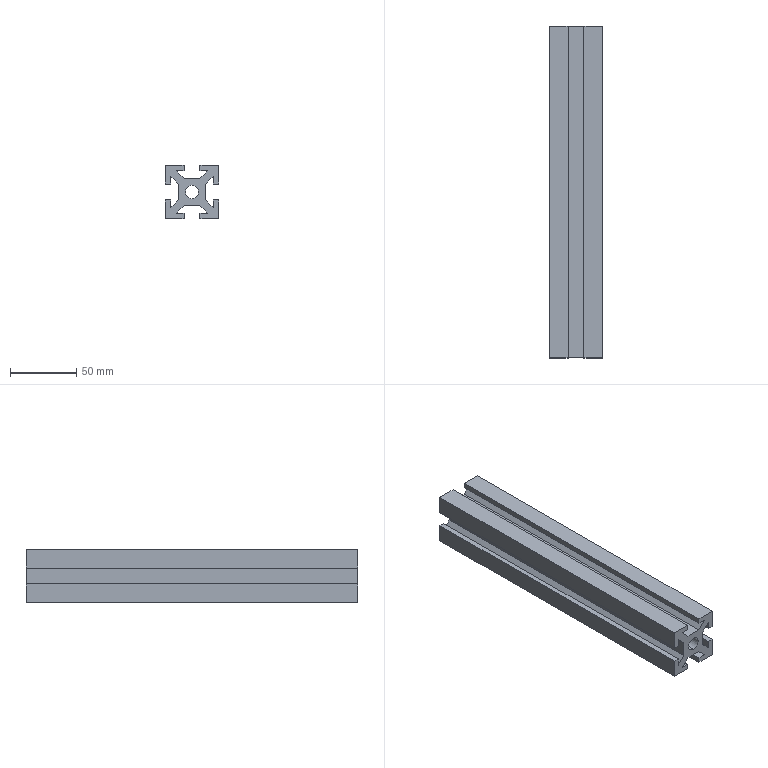Part | SolidWorks | features Extrusion 1 | 1 solid | 40 faces | box 40 x 250 x 40 mm | volume 227277 mm3 | plane 38 | cylinder 2 | commonest cylinder face diameters 10 x2
STEP:
#1=CARTESIAN_POINT('',(0.,250.,-5.));
#2=VERTEX_POINT('',#1);
#3=CARTESIAN_POINT('',(0.,250.,5.));
#4=VERTEX_POINT('',#3);
#5=CARTESIAN_POINT('',(0.,250.,0.));
#6=DIRECTION('',(0.,1.,0.));
#7=DIRECTION('',(0.,0.,1.));
#8=AXIS2_PLACEMENT_3D('',#5,#6,#7);
#9=CIRCLE('',#8,5.);
#10=EDGE_CURVE('',#2,#4,#9,.T.);
#11=ORIENTED_EDGE('',*,*,#10,.T.);
#12=CARTESIAN_POINT('',(0.,0.,5.));
#13=VERTEX_POINT('',#12);
#14=CARTESIAN_POINT('',(0.,250.,5.));
#15=DIRECTION('',(0.,-1.,0.));
#16=VECTOR('',#15,1000.);
#17=LINE('',#14,#16);
#18=EDGE_CURVE('',#4,#13,#17,.T.);
#19=ORIENTED_EDGE('',*,*,#18,.T.);
#20=CARTESIAN_POINT('',(0.,0.,-5.));
#21=VERTEX_POINT('',#20);
#22=CARTESIAN_POINT('',(0.,0.,0.));
#23=DIRECTION('',(0.,1.,0.));
#24=DIRECTION('',(0.,0.,1.));
#25=AXIS2_PLACEMENT_3D('',#22,#23,#24);
#26=CIRCLE('',#25,5.);
#27=EDGE_CURVE('',#21,#13,#26,.T.);
#28=ORIENTED_EDGE('',*,*,#27,.F.);
#29=CARTESIAN_POINT('',(0.,250.,-5.));
#30=DIRECTION('',(0.,-1.,0.));
#31=VECTOR('',#30,1000.);
#32=LINE('',#29,#31);
#33=EDGE_CURVE('',#2,#21,#32,.T.);
#34=ORIENTED_EDGE('',*,*,#33,.F.);
#35=EDGE_LOOP('',(#11,#19,#28,#34));
#36=FACE_OUTER_BOUND('',#35,.T.);
#37=CARTESIAN_POINT('',(0.,250.,0.));
#38=DIRECTION('',(0.,-1.,0.));
#39=DIRECTION('',(0.,0.,-1.));
#40=AXIS2_PLACEMENT_3D('',#37,#38,#39);
#41=CYLINDRICAL_SURFACE('',#40,5.);
#42=ADVANCED_FACE('',(#36),#41,.F.);
#43=CARTESIAN_POINT('',(6.,250.,20.));
#44=VERTEX_POINT('',#43);
#45=CARTESIAN_POINT('',(20.,250.,20.));
#46=VERTEX_POINT('',#45);
#47=CARTESIAN_POINT('',(6.,250.,20.));
#48=DIRECTION('',(1.,0.,0.));
#49=VECTOR('',#48,1000.);
#50=LINE('',#47,#49);
#51=EDGE_CURVE('',#44,#46,#50,.T.);
#52=ORIENTED_EDGE('',*,*,#51,.T.);
#53=CARTESIAN_POINT('',(20.,250.,6.));
#54=VERTEX_POINT('',#53);
#55=CARTESIAN_POINT('',(20.,250.,6.));
#56=DIRECTION('',(0.,0.,-1.));
#57=VECTOR('',#56,1000.);
#58=LINE('',#55,#57);
#59=EDGE_CURVE('',#46,#54,#58,.T.);
#60=ORIENTED_EDGE('',*,*,#59,.T.);
#61=CARTESIAN_POINT('',(16.,250.,6.));
#62=VERTEX_POINT('',#61);
#63=CARTESIAN_POINT('',(16.,250.,6.));
#64=DIRECTION('',(-1.,0.,0.));
#65=VECTOR('',#64,1000.);
#66=LINE('',#63,#65);
#67=EDGE_CURVE('',#54,#62,#66,.T.);
#68=ORIENTED_EDGE('',*,*,#67,.T.);
#69=CARTESIAN_POINT('',(16.,250.,11.757));
#70=VERTEX_POINT('',#69);
#71=CARTESIAN_POINT('',(16.,250.,11.757));
#72=DIRECTION('',(0.,0.,1.));
#73=VECTOR('',#72,1000.);
#74=LINE('',#71,#73);
#75=EDGE_CURVE('',#62,#70,#74,.T.);
#76=ORIENTED_EDGE('',*,*,#75,.T.);
#77=CARTESIAN_POINT('',(10.,250.,5.757));
#78=VERTEX_POINT('',#77);
#79=CARTESIAN_POINT('',(10.,250.,5.757));
#80=DIRECTION('',(-0.7071,0.,-0.7071));
#81=VECTOR('',#80,1000.);
#82=LINE('',#79,#81);
#83=EDGE_CURVE('',#70,#78,#82,.T.);
#84=ORIENTED_EDGE('',*,*,#83,.T.);
#85=CARTESIAN_POINT('',(10.,250.,-5.757));
#86=VERTEX_POINT('',#85);
#87=CARTESIAN_POINT('',(10.,250.,5.757));
#88=DIRECTION('',(0.,0.,-1.));
#89=VECTOR('',#88,1000.);
#90=LINE('',#87,#89);
#91=EDGE_CURVE('',#78,#86,#90,.T.);
#92=ORIENTED_EDGE('',*,*,#91,.T.);
#93=CARTESIAN_POINT('',(16.,250.,-11.757));
#94=VERTEX_POINT('',#93);
#95=CARTESIAN_POINT('',(16.,250.,-11.757));
#96=DIRECTION('',(0.7071,0.,-0.7071));
#97=VECTOR('',#96,1000.);
#98=LINE('',#95,#97);
#99=EDGE_CURVE('',#86,#94,#98,.T.);
#100=ORIENTED_EDGE('',*,*,#99,.T.);
#101=CARTESIAN_POINT('',(16.,250.,-6.));
#102=VERTEX_POINT('',#101);
#103=CARTESIAN_POINT('',(16.,250.,-6.));
#104=DIRECTION('',(0.,0.,1.));
#105=VECTOR('',#104,1000.);
#106=LINE('',#103,#105);
#107=EDGE_CURVE('',#94,#102,#106,.T.);
#108=ORIENTED_EDGE('',*,*,#107,.T.);
#109=CARTESIAN_POINT('',(20.,250.,-6.));
#110=VERTEX_POINT('',#109);
#111=CARTESIAN_POINT('',(20.,250.,-6.));
#112=DIRECTION('',(1.,0.,0.));
#113=VECTOR('',#112,1000.);
#114=LINE('',#111,#113);
#115=EDGE_CURVE('',#102,#110,#114,.T.);
#116=ORIENTED_EDGE('',*,*,#115,.T.);
#117=CARTESIAN_POINT('',(20.,250.,-20.));
#118=VERTEX_POINT('',#117);
#119=CARTESIAN_POINT('',(20.,250.,-20.));
#120=DIRECTION('',(0.,0.,-1.));
#121=VECTOR('',#120,1000.);
#122=LINE('',#119,#121);
#123=EDGE_CURVE('',#110,#118,#122,.T.);
#124=ORIENTED_EDGE('',*,*,#123,.T.);
#125=CARTESIAN_POINT('',(6.,250.,-20.));
#126=VERTEX_POINT('',#125);
#127=CARTESIAN_POINT('',(6.,250.,-20.));
#128=DIRECTION('',(-1.,0.,0.));
#129=VECTOR('',#128,1000.);
#130=LINE('',#127,#129);
#131=EDGE_CURVE('',#118,#126,#130,.T.);
#132=ORIENTED_EDGE('',*,*,#131,.T.);
#133=CARTESIAN_POINT('',(6.,250.,-16.));
#134=VERTEX_POINT('',#133);
#135=CARTESIAN_POINT('',(6.,250.,-16.));
#136=DIRECTION('',(0.,0.,1.));
#137=VECTOR('',#136,1000.);
#138=LINE('',#135,#137);
#139=EDGE_CURVE('',#126,#134,#138,.T.);
#140=ORIENTED_EDGE('',*,*,#139,.T.);
#141=CARTESIAN_POINT('',(11.757,250.,-16.));
#142=VERTEX_POINT('',#141);
#143=CARTESIAN_POINT('',(11.757,250.,-16.));
#144=DIRECTION('',(1.,0.,0.));
#145=VECTOR('',#144,1000.);
#146=LINE('',#143,#145);
#147=EDGE_CURVE('',#134,#142,#146,.T.);
#148=ORIENTED_EDGE('',*,*,#147,.T.);
#149=CARTESIAN_POINT('',(5.757,250.,-10.));
#150=VERTEX_POINT('',#149);
#151=CARTESIAN_POINT('',(5.757,250.,-10.));
#152=DIRECTION('',(-0.7071,0.,0.7071));
#153=VECTOR('',#152,1000.);
#154=LINE('',#151,#153);
#155=EDGE_CURVE('',#142,#150,#154,.T.);
#156=ORIENTED_EDGE('',*,*,#155,.T.);
#157=CARTESIAN_POINT('',(-5.757,250.,-10.));
#158=VERTEX_POINT('',#157);
#159=CARTESIAN_POINT('',(-5.757,250.,-10.));
#160=DIRECTION('',(-1.,0.,0.));
#161=VECTOR('',#160,1000.);
#162=LINE('',#159,#161);
#163=EDGE_CURVE('',#150,#158,#162,.T.);
#164=ORIENTED_EDGE('',*,*,#163,.T.);
#165=CARTESIAN_POINT('',(-11.757,250.,-16.));
#166=VERTEX_POINT('',#165);
#167=CARTESIAN_POINT('',(-11.757,250.,-16.));
#168=DIRECTION('',(-0.7071,0.,-0.7071));
#169=VECTOR('',#168,1000.);
#170=LINE('',#167,#169);
#171=EDGE_CURVE('',#158,#166,#170,.T.);
#172=ORIENTED_EDGE('',*,*,#171,.T.);
#173=CARTESIAN_POINT('',(-6.,250.,-16.));
#174=VERTEX_POINT('',#173);
#175=CARTESIAN_POINT('',(-6.,250.,-16.));
#176=DIRECTION('',(1.,0.,0.));
#177=VECTOR('',#176,1000.);
#178=LINE('',#175,#177);
#179=EDGE_CURVE('',#166,#174,#178,.T.);
#180=ORIENTED_EDGE('',*,*,#179,.T.);
#181=CARTESIAN_POINT('',(-6.,250.,-20.));
#182=VERTEX_POINT('',#181);
#183=CARTESIAN_POINT('',(-6.,250.,-20.));
#184=DIRECTION('',(0.,0.,-1.));
#185=VECTOR('',#184,1000.);
#186=LINE('',#183,#185);
#187=EDGE_CURVE('',#174,#182,#186,.T.);
#188=ORIENTED_EDGE('',*,*,#187,.T.);
#189=CARTESIAN_POINT('',(-20.,250.,-20.));
#190=VERTEX_POINT('',#189);
#191=CARTESIAN_POINT('',(-20.,250.,-20.));
#192=DIRECTION('',(-1.,0.,0.));
#193=VECTOR('',#192,1000.);
#194=LINE('',#191,#193);
#195=EDGE_CURVE('',#182,#190,#194,.T.);
#196=ORIENTED_EDGE('',*,*,#195,.T.);
#197=CARTESIAN_POINT('',(-20.,250.,-6.));
#198=VERTEX_POINT('',#197);
#199=CARTESIAN_POINT('',(-20.,250.,-20.));
#200=DIRECTION('',(0.,0.,1.));
#201=VECTOR('',#200,1000.);
#202=LINE('',#199,#201);
#203=EDGE_CURVE('',#190,#198,#202,.T.);
#204=ORIENTED_EDGE('',*,*,#203,.T.);
#205=CARTESIAN_POINT('',(-16.,250.,-6.));
#206=VERTEX_POINT('',#205);
#207=CARTESIAN_POINT('',(-16.,250.,-6.));
#208=DIRECTION('',(1.,0.,0.));
#209=VECTOR('',#208,1000.);
#210=LINE('',#207,#209);
#211=EDGE_CURVE('',#198,#206,#210,.T.);
#212=ORIENTED_EDGE('',*,*,#211,.T.);
#213=CARTESIAN_POINT('',(-16.,250.,-11.757));
#214=VERTEX_POINT('',#213);
#215=CARTESIAN_POINT('',(-16.,250.,-11.757));
#216=DIRECTION('',(0.,0.,-1.));
#217=VECTOR('',#216,1000.);
#218=LINE('',#215,#217);
#219=EDGE_CURVE('',#206,#214,#218,.T.);
#220=ORIENTED_EDGE('',*,*,#219,.T.);
#221=CARTESIAN_POINT('',(-10.,250.,-5.757));
#222=VERTEX_POINT('',#221);
#223=CARTESIAN_POINT('',(-10.,250.,-5.757));
#224=DIRECTION('',(0.7071,0.,0.7071));
#225=VECTOR('',#224,1000.);
#226=LINE('',#223,#225);
#227=EDGE_CURVE('',#214,#222,#226,.T.);
#228=ORIENTED_EDGE('',*,*,#227,.T.);
#229=CARTESIAN_POINT('',(-10.,250.,5.757));
#230=VERTEX_POINT('',#229);
#231=CARTESIAN_POINT('',(-10.,250.,5.757));
#232=DIRECTION('',(0.,0.,1.));
#233=VECTOR('',#232,1000.);
#234=LINE('',#231,#233);
#235=EDGE_CURVE('',#222,#230,#234,.T.);
#236=ORIENTED_EDGE('',*,*,#235,.T.);
#237=CARTESIAN_POINT('',(-16.,250.,11.757));
#238=VERTEX_POINT('',#237);
#239=CARTESIAN_POINT('',(-16.,250.,11.757));
#240=DIRECTION('',(-0.7071,0.,0.7071));
#241=VECTOR('',#240,1000.);
#242=LINE('',#239,#241);
#243=EDGE_CURVE('',#230,#238,#242,.T.);
#244=ORIENTED_EDGE('',*,*,#243,.T.);
#245=CARTESIAN_POINT('',(-16.,250.,6.));
#246=VERTEX_POINT('',#245);
#247=CARTESIAN_POINT('',(-16.,250.,6.));
#248=DIRECTION('',(0.,0.,-1.));
#249=VECTOR('',#248,1000.);
#250=LINE('',#247,#249);
#251=EDGE_CURVE('',#238,#246,#250,.T.);
#252=ORIENTED_EDGE('',*,*,#251,.T.);
#253=CARTESIAN_POINT('',(-20.,250.,6.));
#254=VERTEX_POINT('',#253);
#255=CARTESIAN_POINT('',(-20.,250.,6.));
#256=DIRECTION('',(-1.,0.,0.));
#257=VECTOR('',#256,1000.);
#258=LINE('',#255,#257);
#259=EDGE_CURVE('',#246,#254,#258,.T.);
#260=ORIENTED_EDGE('',*,*,#259,.T.);
#261=CARTESIAN_POINT('',(-20.,250.,20.));
#262=VERTEX_POINT('',#261);
#263=CARTESIAN_POINT('',(-20.,250.,6.));
#264=DIRECTION('',(0.,0.,1.));
#265=VECTOR('',#264,1000.);
#266=LINE('',#263,#265);
#267=EDGE_CURVE('',#254,#262,#266,.T.);
#268=ORIENTED_EDGE('',*,*,#267,.T.);
#269=CARTESIAN_POINT('',(-6.,250.,20.));
#270=VERTEX_POINT('',#269);
#271=CARTESIAN_POINT('',(-20.,250.,20.));
#272=DIRECTION('',(1.,0.,0.));
#273=VECTOR('',#272,1000.);
#274=LINE('',#271,#273);
#275=EDGE_CURVE('',#262,#270,#274,.T.);
#276=ORIENTED_EDGE('',*,*,#275,.T.);
#277=CARTESIAN_POINT('',(-6.,250.,16.));
#278=VERTEX_POINT('',#277);
#279=CARTESIAN_POINT('',(-6.,250.,16.));
#280=DIRECTION('',(0.,0.,-1.));
#281=VECTOR('',#280,1000.);
#282=LINE('',#279,#281);
#283=EDGE_CURVE('',#270,#278,#282,.T.);
#284=ORIENTED_EDGE('',*,*,#283,.T.);
#285=CARTESIAN_POINT('',(-11.757,250.,16.));
#286=VERTEX_POINT('',#285);
#287=CARTESIAN_POINT('',(-11.757,250.,16.));
#288=DIRECTION('',(-1.,0.,0.));
#289=VECTOR('',#288,1000.);
#290=LINE('',#287,#289);
#291=EDGE_CURVE('',#278,#286,#290,.T.);
#292=ORIENTED_EDGE('',*,*,#291,.T.);
#293=CARTESIAN_POINT('',(-5.757,250.,10.));
#294=VERTEX_POINT('',#293);
#295=CARTESIAN_POINT('',(-5.757,250.,10.));
#296=DIRECTION('',(0.7071,0.,-0.7071));
#297=VECTOR('',#296,1000.);
#298=LINE('',#295,#297);
#299=EDGE_CURVE('',#286,#294,#298,.T.);
#300=ORIENTED_EDGE('',*,*,#299,.T.);
#301=CARTESIAN_POINT('',(5.757,250.,10.));
#302=VERTEX_POINT('',#301);
#303=CARTESIAN_POINT('',(-5.757,250.,10.));
#304=DIRECTION('',(1.,0.,0.));
#305=VECTOR('',#304,1000.);
#306=LINE('',#303,#305);
#307=EDGE_CURVE('',#294,#302,#306,.T.);
#308=ORIENTED_EDGE('',*,*,#307,.T.);
#309=CARTESIAN_POINT('',(11.757,250.,16.));
#310=VERTEX_POINT('',#309);
#311=CARTESIAN_POINT('',(11.757,250.,16.));
#312=DIRECTION('',(0.7071,0.,0.7071));
#313=VECTOR('',#312,1000.);
#314=LINE('',#311,#313);
#315=EDGE_CURVE('',#302,#310,#314,.T.);
#316=ORIENTED_EDGE('',*,*,#315,.T.);
#317=CARTESIAN_POINT('',(6.,250.,16.));
#318=VERTEX_POINT('',#317);
#319=CARTESIAN_POINT('',(6.,250.,16.));
#320=DIRECTION('',(-1.,0.,0.));
#321=VECTOR('',#320,1000.);
#322=LINE('',#319,#321);
#323=EDGE_CURVE('',#310,#318,#322,.T.);
#324=ORIENTED_EDGE('',*,*,#323,.T.);
#325=CARTESIAN_POINT('',(6.,250.,20.));
#326=DIRECTION('',(0.,0.,1.));
#327=VECTOR('',#326,1000.);
#328=LINE('',#325,#327);
#329=EDGE_CURVE('',#318,#44,#328,.T.);
#330=ORIENTED_EDGE('',*,*,#329,.T.);
#331=EDGE_LOOP('',(#52,#60,#68,#76,#84,#92,#100,#108,#116,#124,#132,#140,#148,#156,#164,#172,#180,#188,#196,#204,#212,#220,#228,#236,#244,#252,#260,#268,#276,#284,#292,#300,#308,#316,#324,#330));
#332=FACE_OUTER_BOUND('',#331,.T.);
#333=ORIENTED_EDGE('',*,*,#10,.F.);
#334=CARTESIAN_POINT('',(0.,250.,0.));
#335=DIRECTION('',(0.,1.,0.));
#336=DIRECTION('',(0.,0.,1.));
#337=AXIS2_PLACEMENT_3D('',#334,#335,#336);
#338=CIRCLE('',#337,5.);
#339=EDGE_CURVE('',#4,#2,#338,.T.);
#340=ORIENTED_EDGE('',*,*,#339,.F.);
#341=EDGE_LOOP('',(#333,#340));
#342=FACE_BOUND('',#341,.T.);
#343=CARTESIAN_POINT('',(0.,250.,0.));
#344=DIRECTION('',(0.,-1.,0.));
#345=DIRECTION('',(0.,0.,-1.));
#346=AXIS2_PLACEMENT_3D('',#343,#344,#345);
#347=PLANE('',#346);
#348=ADVANCED_FACE('',(#332,#342),#347,.F.);
#349=CARTESIAN_POINT('',(6.,0.,20.));
#350=VERTEX_POINT('',#349);
#351=CARTESIAN_POINT('',(20.,0.,20.));
#352=VERTEX_POINT('',#351);
#353=CARTESIAN_POINT('',(6.,0.,20.));
#354=DIRECTION('',(1.,0.,0.));
#355=VECTOR('',#354,1000.);
#356=LINE('',#353,#355);
#357=EDGE_CURVE('',#350,#352,#356,.T.);
#358=ORIENTED_EDGE('',*,*,#357,.F.);
#359=CARTESIAN_POINT('',(6.,0.,16.));
#360=VERTEX_POINT('',#359);
#361=CARTESIAN_POINT('',(6.,0.,20.));
#362=DIRECTION('',(0.,0.,1.));
#363=VECTOR('',#362,1000.);
#364=LINE('',#361,#363);
#365=EDGE_CURVE('',#360,#350,#364,.T.);
#366=ORIENTED_EDGE('',*,*,#365,.F.);
#367=CARTESIAN_POINT('',(11.757,0.,16.));
#368=VERTEX_POINT('',#367);
#369=CARTESIAN_POINT('',(6.,0.,16.));
#370=DIRECTION('',(-1.,0.,0.));
#371=VECTOR('',#370,1000.);
#372=LINE('',#369,#371);
#373=EDGE_CURVE('',#368,#360,#372,.T.);
#374=ORIENTED_EDGE('',*,*,#373,.F.);
#375=CARTESIAN_POINT('',(5.757,0.,10.));
#376=VERTEX_POINT('',#375);
#377=CARTESIAN_POINT('',(11.757,0.,16.));
#378=DIRECTION('',(0.7071,0.,0.7071));
#379=VECTOR('',#378,1000.);
#380=LINE('',#377,#379);
#381=EDGE_CURVE('',#376,#368,#380,.T.);
#382=ORIENTED_EDGE('',*,*,#381,.F.);
#383=CARTESIAN_POINT('',(-5.757,0.,10.));
#384=VERTEX_POINT('',#383);
#385=CARTESIAN_POINT('',(-5.757,0.,10.));
#386=DIRECTION('',(1.,0.,0.));
#387=VECTOR('',#386,1000.);
#388=LINE('',#385,#387);
#389=EDGE_CURVE('',#384,#376,#388,.T.);
#390=ORIENTED_EDGE('',*,*,#389,.F.);
#391=CARTESIAN_POINT('',(-11.757,0.,16.));
#392=VERTEX_POINT('',#391);
#393=CARTESIAN_POINT('',(-5.757,0.,10.));
#394=DIRECTION('',(0.7071,0.,-0.7071));
#395=VECTOR('',#394,1000.);
#396=LINE('',#393,#395);
#397=EDGE_CURVE('',#392,#384,#396,.T.);
#398=ORIENTED_EDGE('',*,*,#397,.F.);
#399=CARTESIAN_POINT('',(-6.,0.,16.));
#400=VERTEX_POINT('',#399);
#401=CARTESIAN_POINT('',(-11.757,0.,16.));
#402=DIRECTION('',(-1.,0.,0.));
#403=VECTOR('',#402,1000.);
#404=LINE('',#401,#403);
#405=EDGE_CURVE('',#400,#392,#404,.T.);
#406=ORIENTED_EDGE('',*,*,#405,.F.);
#407=CARTESIAN_POINT('',(-6.,0.,20.));
#408=VERTEX_POINT('',#407);
#409=CARTESIAN_POINT('',(-6.,0.,16.));
#410=DIRECTION('',(0.,0.,-1.));
#411=VECTOR('',#410,1000.);
#412=LINE('',#409,#411);
#413=EDGE_CURVE('',#408,#400,#412,.T.);
#414=ORIENTED_EDGE('',*,*,#413,.F.);
#415=CARTESIAN_POINT('',(-20.,0.,20.));
#416=VERTEX_POINT('',#415);
#417=CARTESIAN_POINT('',(-20.,0.,20.));
#418=DIRECTION('',(1.,0.,0.));
#419=VECTOR('',#418,1000.);
#420=LINE('',#417,#419);
#421=EDGE_CURVE('',#416,#408,#420,.T.);
#422=ORIENTED_EDGE('',*,*,#421,.F.);
#423=CARTESIAN_POINT('',(-20.,0.,6.));
#424=VERTEX_POINT('',#423);
#425=CARTESIAN_POINT('',(-20.,0.,6.));
#426=DIRECTION('',(0.,0.,1.));
#427=VECTOR('',#426,1000.);
#428=LINE('',#425,#427);
#429=EDGE_CURVE('',#424,#416,#428,.T.);
#430=ORIENTED_EDGE('',*,*,#429,.F.);
#431=CARTESIAN_POINT('',(-16.,0.,6.));
#432=VERTEX_POINT('',#431);
#433=CARTESIAN_POINT('',(-20.,0.,6.));
#434=DIRECTION('',(-1.,0.,0.));
#435=VECTOR('',#434,1000.);
#436=LINE('',#433,#435);
#437=EDGE_CURVE('',#432,#424,#436,.T.);
#438=ORIENTED_EDGE('',*,*,#437,.F.);
#439=CARTESIAN_POINT('',(-16.,0.,11.757));
#440=VERTEX_POINT('',#439);
#441=CARTESIAN_POINT('',(-16.,0.,6.));
#442=DIRECTION('',(0.,0.,-1.));
#443=VECTOR('',#442,1000.);
#444=LINE('',#441,#443);
#445=EDGE_CURVE('',#440,#432,#444,.T.);
#446=ORIENTED_EDGE('',*,*,#445,.F.);
#447=CARTESIAN_POINT('',(-10.,0.,5.757));
#448=VERTEX_POINT('',#447);
#449=CARTESIAN_POINT('',(-16.,0.,11.757));
#450=DIRECTION('',(-0.7071,0.,0.7071));
#451=VECTOR('',#450,1000.);
#452=LINE('',#449,#451);
#453=EDGE_CURVE('',#448,#440,#452,.T.);
#454=ORIENTED_EDGE('',*,*,#453,.F.);
#455=CARTESIAN_POINT('',(-10.,0.,-5.757));
#456=VERTEX_POINT('',#455);
#457=CARTESIAN_POINT('',(-10.,0.,5.757));
#458=DIRECTION('',(0.,0.,1.));
#459=VECTOR('',#458,1000.);
#460=LINE('',#457,#459);
#461=EDGE_CURVE('',#456,#448,#460,.T.);
#462=ORIENTED_EDGE('',*,*,#461,.F.);
#463=CARTESIAN_POINT('',(-16.,0.,-11.757));
#464=VERTEX_POINT('',#463);
#465=CARTESIAN_POINT('',(-10.,0.,-5.757));
#466=DIRECTION('',(0.7071,0.,0.7071));
#467=VECTOR('',#466,1000.);
#468=LINE('',#465,#467);
#469=EDGE_CURVE('',#464,#456,#468,.T.);
#470=ORIENTED_EDGE('',*,*,#469,.F.);
#471=CARTESIAN_POINT('',(-16.,0.,-6.));
#472=VERTEX_POINT('',#471);
#473=CARTESIAN_POINT('',(-16.,0.,-11.757));
#474=DIRECTION('',(0.,0.,-1.));
#475=VECTOR('',#474,1000.);
#476=LINE('',#473,#475);
#477=EDGE_CURVE('',#472,#464,#476,.T.);
#478=ORIENTED_EDGE('',*,*,#477,.F.);
#479=CARTESIAN_POINT('',(-20.,0.,-6.));
#480=VERTEX_POINT('',#479);
#481=CARTESIAN_POINT('',(-16.,0.,-6.));
#482=DIRECTION('',(1.,0.,0.));
#483=VECTOR('',#482,1000.);
#484=LINE('',#481,#483);
#485=EDGE_CURVE('',#480,#472,#484,.T.);
#486=ORIENTED_EDGE('',*,*,#485,.F.);
#487=CARTESIAN_POINT('',(-20.,0.,-20.));
#488=VERTEX_POINT('',#487);
#489=CARTESIAN_POINT('',(-20.,0.,-20.));
#490=DIRECTION('',(0.,0.,1.));
#491=VECTOR('',#490,1000.);
#492=LINE('',#489,#491);
#493=EDGE_CURVE('',#488,#480,#492,.T.);
#494=ORIENTED_EDGE('',*,*,#493,.F.);
#495=CARTESIAN_POINT('',(-6.,0.,-20.));
#496=VERTEX_POINT('',#495);
#497=CARTESIAN_POINT('',(-20.,0.,-20.));
#498=DIRECTION('',(-1.,0.,0.));
#499=VECTOR('',#498,1000.);
#500=LINE('',#497,#499);
#501=EDGE_CURVE('',#496,#488,#500,.T.);
#502=ORIENTED_EDGE('',*,*,#501,.F.);
#503=CARTESIAN_POINT('',(-6.,0.,-16.));
#504=VERTEX_POINT('',#503);
#505=CARTESIAN_POINT('',(-6.,0.,-20.));
#506=DIRECTION('',(0.,0.,-1.));
#507=VECTOR('',#506,1000.);
#508=LINE('',#505,#507);
#509=EDGE_CURVE('',#504,#496,#508,.T.);
#510=ORIENTED_EDGE('',*,*,#509,.F.);
#511=CARTESIAN_POINT('',(-11.757,0.,-16.));
#512=VERTEX_POINT('',#511);
#513=CARTESIAN_POINT('',(-6.,0.,-16.));
#514=DIRECTION('',(1.,0.,0.));
#515=VECTOR('',#514,1000.);
#516=LINE('',#513,#515);
#517=EDGE_CURVE('',#512,#504,#516,.T.);
#518=ORIENTED_EDGE('',*,*,#517,.F.);
#519=CARTESIAN_POINT('',(-5.757,0.,-10.));
#520=VERTEX_POINT('',#519);
#521=CARTESIAN_POINT('',(-11.757,0.,-16.));
#522=DIRECTION('',(-0.7071,0.,-0.7071));
#523=VECTOR('',#522,1000.);
#524=LINE('',#521,#523);
#525=EDGE_CURVE('',#520,#512,#524,.T.);
#526=ORIENTED_EDGE('',*,*,#525,.F.);
#527=CARTESIAN_POINT('',(5.757,0.,-10.));
#528=VERTEX_POINT('',#527);
#529=CARTESIAN_POINT('',(-5.757,0.,-10.));
#530=DIRECTION('',(-1.,0.,0.));
#531=VECTOR('',#530,1000.);
#532=LINE('',#529,#531);
#533=EDGE_CURVE('',#528,#520,#532,.T.);
#534=ORIENTED_EDGE('',*,*,#533,.F.);
#535=CARTESIAN_POINT('',(11.757,0.,-16.));
#536=VERTEX_POINT('',#535);
#537=CARTESIAN_POINT('',(5.757,0.,-10.));
#538=DIRECTION('',(-0.7071,0.,0.7071));
#539=VECTOR('',#538,1000.);
#540=LINE('',#537,#539);
#541=EDGE_CURVE('',#536,#528,#540,.T.);
#542=ORIENTED_EDGE('',*,*,#541,.F.);
#543=CARTESIAN_POINT('',(6.,0.,-16.));
#544=VERTEX_POINT('',#543);
#545=CARTESIAN_POINT('',(11.757,0.,-16.));
#546=DIRECTION('',(1.,0.,0.));
#547=VECTOR('',#546,1000.);
#548=LINE('',#545,#547);
#549=EDGE_CURVE('',#544,#536,#548,.T.);
#550=ORIENTED_EDGE('',*,*,#549,.F.);
#551=CARTESIAN_POINT('',(6.,0.,-20.));
#552=VERTEX_POINT('',#551);
#553=CARTESIAN_POINT('',(6.,0.,-16.));
#554=DIRECTION('',(0.,0.,1.));
#555=VECTOR('',#554,1000.);
#556=LINE('',#553,#555);
#557=EDGE_CURVE('',#552,#544,#556,.T.);
#558=ORIENTED_EDGE('',*,*,#557,.F.);
#559=CARTESIAN_POINT('',(20.,0.,-20.));
#560=VERTEX_POINT('',#559);
#561=CARTESIAN_POINT('',(6.,0.,-20.));
#562=DIRECTION('',(-1.,0.,0.));
#563=VECTOR('',#562,1000.);
#564=LINE('',#561,#563);
#565=EDGE_CURVE('',#560,#552,#564,.T.);
#566=ORIENTED_EDGE('',*,*,#565,.F.);
#567=CARTESIAN_POINT('',(20.,0.,-6.));
#568=VERTEX_POINT('',#567);
#569=CARTESIAN_POINT('',(20.,0.,-20.));
#570=DIRECTION('',(0.,0.,-1.));
#571=VECTOR('',#570,1000.);
#572=LINE('',#569,#571);
#573=EDGE_CURVE('',#568,#560,#572,.T.);
#574=ORIENTED_EDGE('',*,*,#573,.F.);
#575=CARTESIAN_POINT('',(16.,0.,-6.));
#576=VERTEX_POINT('',#575);
#577=CARTESIAN_POINT('',(20.,0.,-6.));
#578=DIRECTION('',(1.,0.,0.));
#579=VECTOR('',#578,1000.);
#580=LINE('',#577,#579);
#581=EDGE_CURVE('',#576,#568,#580,.T.);
#582=ORIENTED_EDGE('',*,*,#581,.F.);
#583=CARTESIAN_POINT('',(16.,0.,-11.757));
#584=VERTEX_POINT('',#583);
#585=CARTESIAN_POINT('',(16.,0.,-6.));
#586=DIRECTION('',(0.,0.,1.));
#587=VECTOR('',#586,1000.);
#588=LINE('',#585,#587);
#589=EDGE_CURVE('',#584,#576,#588,.T.);
#590=ORIENTED_EDGE('',*,*,#589,.F.);
#591=CARTESIAN_POINT('',(10.,0.,-5.757));
#592=VERTEX_POINT('',#591);
#593=CARTESIAN_POINT('',(16.,0.,-11.757));
#594=DIRECTION('',(0.7071,0.,-0.7071));
#595=VECTOR('',#594,1000.);
#596=LINE('',#593,#595);
#597=EDGE_CURVE('',#592,#584,#596,.T.);
#598=ORIENTED_EDGE('',*,*,#597,.F.);
#599=CARTESIAN_POINT('',(10.,0.,5.757));
#600=VERTEX_POINT('',#599);
#601=CARTESIAN_POINT('',(10.,0.,5.757));
#602=DIRECTION('',(0.,0.,-1.));
#603=VECTOR('',#602,1000.);
#604=LINE('',#601,#603);
#605=EDGE_CURVE('',#600,#592,#604,.T.);
#606=ORIENTED_EDGE('',*,*,#605,.F.);
#607=CARTESIAN_POINT('',(16.,0.,11.757));
#608=VERTEX_POINT('',#607);
#609=CARTESIAN_POINT('',(10.,0.,5.757));
#610=DIRECTION('',(-0.7071,0.,-0.7071));
#611=VECTOR('',#610,1000.);
#612=LINE('',#609,#611);
#613=EDGE_CURVE('',#608,#600,#612,.T.);
#614=ORIENTED_EDGE('',*,*,#613,.F.);
#615=CARTESIAN_POINT('',(16.,0.,6.));
#616=VERTEX_POINT('',#615);
#617=CARTESIAN_POINT('',(16.,0.,11.757));
#618=DIRECTION('',(0.,0.,1.));
#619=VECTOR('',#618,1000.);
#620=LINE('',#617,#619);
#621=EDGE_CURVE('',#616,#608,#620,.T.);
#622=ORIENTED_EDGE('',*,*,#621,.F.);
#623=CARTESIAN_POINT('',(20.,0.,6.));
#624=VERTEX_POINT('',#623);
#625=CARTESIAN_POINT('',(16.,0.,6.));
#626=DIRECTION('',(-1.,0.,0.));
#627=VECTOR('',#626,1000.);
#628=LINE('',#625,#627);
#629=EDGE_CURVE('',#624,#616,#628,.T.);
#630=ORIENTED_EDGE('',*,*,#629,.F.);
#631=CARTESIAN_POINT('',(20.,0.,6.));
#632=DIRECTION('',(0.,0.,-1.));
#633=VECTOR('',#632,1000.);
#634=LINE('',#631,#633);
#635=EDGE_CURVE('',#352,#624,#634,.T.);
#636=ORIENTED_EDGE('',*,*,#635,.F.);
#637=EDGE_LOOP('',(#358,#366,#374,#382,#390,#398,#406,#414,#422,#430,#438,#446,#454,#462,#470,#478,#486,#494,#502,#510,#518,#526,#534,#542,#550,#558,#566,#574,#582,#590,#598,#606,#614,#622,#630,#636));
#638=FACE_OUTER_BOUND('',#637,.T.);
#639=ORIENTED_EDGE('',*,*,#27,.T.);
#640=CARTESIAN_POINT('',(0.,0.,0.));
#641=DIRECTION('',(0.,1.,0.));
#642=DIRECTION('',(0.,0.,1.));
#643=AXIS2_PLACEMENT_3D('',#640,#641,#642);
#644=CIRCLE('',#643,5.);
#645=EDGE_CURVE('',#13,#21,#644,.T.);
#646=ORIENTED_EDGE('',*,*,#645,.T.);
#647=EDGE_LOOP('',(#639,#646));
#648=FACE_BOUND('',#647,.T.);
#649=CARTESIAN_POINT('',(0.,0.,0.));
#650=DIRECTION('',(0.,-1.,0.));
#651=DIRECTION('',(0.,0.,-1.));
#652=AXIS2_PLACEMENT_3D('',#649,#650,#651);
#653=PLANE('',#652);
#654=ADVANCED_FACE('',(#638,#648),#653,.T.);
#655=ORIENTED_EDGE('',*,*,#357,.T.);
#656=CARTESIAN_POINT('',(20.,250.,20.));
#657=DIRECTION('',(0.,-1.,0.));
#658=VECTOR('',#657,1000.);
#659=LINE('',#656,#658);
#660=EDGE_CURVE('',#46,#352,#659,.T.);
#661=ORIENTED_EDGE('',*,*,#660,.F.);
#662=ORIENTED_EDGE('',*,*,#51,.F.);
#663=CARTESIAN_POINT('',(6.,250.,20.));
#664=DIRECTION('',(0.,-1.,0.));
#665=VECTOR('',#664,1000.);
#666=LINE('',#663,#665);
#667=EDGE_CURVE('',#44,#350,#666,.T.);
#668=ORIENTED_EDGE('',*,*,#667,.T.);
#669=EDGE_LOOP('',(#655,#661,#662,#668));
#670=FACE_OUTER_BOUND('',#669,.T.);
#671=CARTESIAN_POINT('',(6.,250.,20.));
#672=DIRECTION('',(0.,0.,-1.));
#673=DIRECTION('',(-1.,0.,0.));
#674=AXIS2_PLACEMENT_3D('',#671,#672,#673);
#675=PLANE('',#674);
#676=ADVANCED_FACE('',(#670),#675,.F.);
#677=ORIENTED_EDGE('',*,*,#635,.T.);
#678=CARTESIAN_POINT('',(20.,250.,6.));
#679=DIRECTION('',(0.,-1.,0.));
#680=VECTOR('',#679,1000.);
#681=LINE('',#678,#680);
#682=EDGE_CURVE('',#54,#624,#681,.T.);
#683=ORIENTED_EDGE('',*,*,#682,.F.);
#684=ORIENTED_EDGE('',*,*,#59,.F.);
#685=ORIENTED_EDGE('',*,*,#660,.T.);
#686=EDGE_LOOP('',(#677,#683,#684,#685));
#687=FACE_OUTER_BOUND('',#686,.T.);
#688=CARTESIAN_POINT('',(20.,250.,6.));
#689=DIRECTION('',(-1.,0.,0.));
#690=DIRECTION('',(0.,0.,1.));
#691=AXIS2_PLACEMENT_3D('',#688,#689,#690);
#692=PLANE('',#691);
#693=ADVANCED_FACE('',(#687),#692,.F.);
#694=ORIENTED_EDGE('',*,*,#629,.T.);
#695=CARTESIAN_POINT('',(16.,250.,6.));
#696=DIRECTION('',(0.,-1.,0.));
#697=VECTOR('',#696,1000.);
#698=LINE('',#695,#697);
#699=EDGE_CURVE('',#62,#616,#698,.T.);
#700=ORIENTED_EDGE('',*,*,#699,.F.);
#701=ORIENTED_EDGE('',*,*,#67,.F.);
#702=ORIENTED_EDGE('',*,*,#682,.T.);
#703=EDGE_LOOP('',(#694,#700,#701,#702));
#704=FACE_OUTER_BOUND('',#703,.T.);
#705=CARTESIAN_POINT('',(16.,250.,6.));
#706=DIRECTION('',(0.,0.,1.));
#707=DIRECTION('',(1.,0.,0.));
#708=AXIS2_PLACEMENT_3D('',#705,#706,#707);
#709=PLANE('',#708);
#710=ADVANCED_FACE('',(#704),#709,.F.);
#711=ORIENTED_EDGE('',*,*,#621,.T.);
#712=CARTESIAN_POINT('',(16.,250.,11.757));
#713=DIRECTION('',(0.,-1.,0.));
#714=VECTOR('',#713,1000.);
#715=LINE('',#712,#714);
#716=EDGE_CURVE('',#70,#608,#715,.T.);
#717=ORIENTED_EDGE('',*,*,#716,.F.);
#718=ORIENTED_EDGE('',*,*,#75,.F.);
#719=ORIENTED_EDGE('',*,*,#699,.T.);
#720=EDGE_LOOP('',(#711,#717,#718,#719));
#721=FACE_OUTER_BOUND('',#720,.T.);
#722=CARTESIAN_POINT('',(16.,250.,11.757));
#723=DIRECTION('',(1.,0.,0.));
#724=DIRECTION('',(0.,0.,-1.));
#725=AXIS2_PLACEMENT_3D('',#722,#723,#724);
#726=PLANE('',#725);
#727=ADVANCED_FACE('',(#721),#726,.F.);
#728=ORIENTED_EDGE('',*,*,#613,.T.);
#729=CARTESIAN_POINT('',(10.,250.,5.757));
#730=DIRECTION('',(0.,-1.,0.));
#731=VECTOR('',#730,1000.);
#732=LINE('',#729,#731);
#733=EDGE_CURVE('',#78,#600,#732,.T.);
#734=ORIENTED_EDGE('',*,*,#733,.F.);
#735=ORIENTED_EDGE('',*,*,#83,.F.);
#736=ORIENTED_EDGE('',*,*,#716,.T.);
#737=EDGE_LOOP('',(#728,#734,#735,#736));
#738=FACE_OUTER_BOUND('',#737,.T.);
#739=CARTESIAN_POINT('',(10.,250.,5.757));
#740=DIRECTION('',(-0.7071,0.,0.7071));
#741=DIRECTION('',(0.7071,0.,0.7071));
#742=AXIS2_PLACEMENT_3D('',#739,#740,#741);
#743=PLANE('',#742);
#744=ADVANCED_FACE('',(#738),#743,.F.);
#745=ORIENTED_EDGE('',*,*,#605,.T.);
#746=CARTESIAN_POINT('',(10.,250.,-5.757));
#747=DIRECTION('',(0.,-1.,0.));
#748=VECTOR('',#747,1000.);
#749=LINE('',#746,#748);
#750=EDGE_CURVE('',#86,#592,#749,.T.);
#751=ORIENTED_EDGE('',*,*,#750,.F.);
#752=ORIENTED_EDGE('',*,*,#91,.F.);
#753=ORIENTED_EDGE('',*,*,#733,.T.);
#754=EDGE_LOOP('',(#745,#751,#752,#753));
#755=FACE_OUTER_BOUND('',#754,.T.);
#756=CARTESIAN_POINT('',(10.,250.,5.757));
#757=DIRECTION('',(-1.,0.,0.));
#758=DIRECTION('',(0.,0.,1.));
#759=AXIS2_PLACEMENT_3D('',#756,#757,#758);
#760=PLANE('',#759);
#761=ADVANCED_FACE('',(#755),#760,.F.);
#762=ORIENTED_EDGE('',*,*,#597,.T.);
#763=CARTESIAN_POINT('',(16.,250.,-11.757));
#764=DIRECTION('',(0.,-1.,0.));
#765=VECTOR('',#764,1000.);
#766=LINE('',#763,#765);
#767=EDGE_CURVE('',#94,#584,#766,.T.);
#768=ORIENTED_EDGE('',*,*,#767,.F.);
#769=ORIENTED_EDGE('',*,*,#99,.F.);
#770=ORIENTED_EDGE('',*,*,#750,.T.);
#771=EDGE_LOOP('',(#762,#768,#769,#770));
#772=FACE_OUTER_BOUND('',#771,.T.);
#773=CARTESIAN_POINT('',(16.,250.,-11.757));
#774=DIRECTION('',(-0.7071,0.,-0.7071));
#775=DIRECTION('',(-0.7071,0.,0.7071));
#776=AXIS2_PLACEMENT_3D('',#773,#774,#775);
#777=PLANE('',#776);
#778=ADVANCED_FACE('',(#772),#777,.F.);
#779=ORIENTED_EDGE('',*,*,#589,.T.);
#780=CARTESIAN_POINT('',(16.,250.,-6.));
#781=DIRECTION('',(0.,-1.,0.));
#782=VECTOR('',#781,1000.);
#783=LINE('',#780,#782);
#784=EDGE_CURVE('',#102,#576,#783,.T.);
#785=ORIENTED_EDGE('',*,*,#784,.F.);
#786=ORIENTED_EDGE('',*,*,#107,.F.);
#787=ORIENTED_EDGE('',*,*,#767,.T.);
#788=EDGE_LOOP('',(#779,#785,#786,#787));
#789=FACE_OUTER_BOUND('',#788,.T.);
#790=CARTESIAN_POINT('',(16.,250.,-6.));
#791=DIRECTION('',(1.,0.,0.));
#792=DIRECTION('',(0.,0.,-1.));
#793=AXIS2_PLACEMENT_3D('',#790,#791,#792);
#794=PLANE('',#793);
#795=ADVANCED_FACE('',(#789),#794,.F.);
#796=ORIENTED_EDGE('',*,*,#581,.T.);
#797=CARTESIAN_POINT('',(20.,250.,-6.));
#798=DIRECTION('',(0.,-1.,0.));
#799=VECTOR('',#798,1000.);
#800=LINE('',#797,#799);
#801=EDGE_CURVE('',#110,#568,#800,.T.);
#802=ORIENTED_EDGE('',*,*,#801,.F.);
#803=ORIENTED_EDGE('',*,*,#115,.F.);
#804=ORIENTED_EDGE('',*,*,#784,.T.);
#805=EDGE_LOOP('',(#796,#802,#803,#804));
#806=FACE_OUTER_BOUND('',#805,.T.);
#807=CARTESIAN_POINT('',(20.,250.,-6.));
#808=DIRECTION('',(0.,0.,-1.));
#809=DIRECTION('',(-1.,0.,0.));
#810=AXIS2_PLACEMENT_3D('',#807,#808,#809);
#811=PLANE('',#810);
#812=ADVANCED_FACE('',(#806),#811,.F.);
#813=ORIENTED_EDGE('',*,*,#573,.T.);
#814=CARTESIAN_POINT('',(20.,250.,-20.));
#815=DIRECTION('',(0.,-1.,0.));
#816=VECTOR('',#815,1000.);
#817=LINE('',#814,#816);
#818=EDGE_CURVE('',#118,#560,#817,.T.);
#819=ORIENTED_EDGE('',*,*,#818,.F.);
#820=ORIENTED_EDGE('',*,*,#123,.F.);
#821=ORIENTED_EDGE('',*,*,#801,.T.);
#822=EDGE_LOOP('',(#813,#819,#820,#821));
#823=FACE_OUTER_BOUND('',#822,.T.);
#824=CARTESIAN_POINT('',(20.,250.,-20.));
#825=DIRECTION('',(-1.,0.,0.));
#826=DIRECTION('',(0.,0.,1.));
#827=AXIS2_PLACEMENT_3D('',#824,#825,#826);
#828=PLANE('',#827);
#829=ADVANCED_FACE('',(#823),#828,.F.);
#830=ORIENTED_EDGE('',*,*,#565,.T.);
#831=CARTESIAN_POINT('',(6.,250.,-20.));
#832=DIRECTION('',(0.,-1.,0.));
#833=VECTOR('',#832,1000.);
#834=LINE('',#831,#833);
#835=EDGE_CURVE('',#126,#552,#834,.T.);
#836=ORIENTED_EDGE('',*,*,#835,.F.);
#837=ORIENTED_EDGE('',*,*,#131,.F.);
#838=ORIENTED_EDGE('',*,*,#818,.T.);
#839=EDGE_LOOP('',(#830,#836,#837,#838));
#840=FACE_OUTER_BOUND('',#839,.T.);
#841=CARTESIAN_POINT('',(6.,250.,-20.));
#842=DIRECTION('',(0.,0.,1.));
#843=DIRECTION('',(1.,0.,0.));
#844=AXIS2_PLACEMENT_3D('',#841,#842,#843);
#845=PLANE('',#844);
#846=ADVANCED_FACE('',(#840),#845,.F.);
#847=ORIENTED_EDGE('',*,*,#557,.T.);
#848=CARTESIAN_POINT('',(6.,250.,-16.));
#849=DIRECTION('',(0.,-1.,0.));
#850=VECTOR('',#849,1000.);
#851=LINE('',#848,#850);
#852=EDGE_CURVE('',#134,#544,#851,.T.);
#853=ORIENTED_EDGE('',*,*,#852,.F.);
#854=ORIENTED_EDGE('',*,*,#139,.F.);
#855=ORIENTED_EDGE('',*,*,#835,.T.);
#856=EDGE_LOOP('',(#847,#853,#854,#855));
#857=FACE_OUTER_BOUND('',#856,.T.);
#858=CARTESIAN_POINT('',(6.,250.,-16.));
#859=DIRECTION('',(1.,0.,0.));
#860=DIRECTION('',(0.,0.,-1.));
#861=AXIS2_PLACEMENT_3D('',#858,#859,#860);
#862=PLANE('',#861);
#863=ADVANCED_FACE('',(#857),#862,.F.);
#864=ORIENTED_EDGE('',*,*,#549,.T.);
#865=CARTESIAN_POINT('',(11.757,250.,-16.));
#866=DIRECTION('',(0.,-1.,0.));
#867=VECTOR('',#866,1000.);
#868=LINE('',#865,#867);
#869=EDGE_CURVE('',#142,#536,#868,.T.);
#870=ORIENTED_EDGE('',*,*,#869,.F.);
#871=ORIENTED_EDGE('',*,*,#147,.F.);
#872=ORIENTED_EDGE('',*,*,#852,.T.);
#873=EDGE_LOOP('',(#864,#870,#871,#872));
#874=FACE_OUTER_BOUND('',#873,.T.);
#875=CARTESIAN_POINT('',(11.757,250.,-16.));
#876=DIRECTION('',(0.,0.,-1.));
#877=DIRECTION('',(-1.,0.,0.));
#878=AXIS2_PLACEMENT_3D('',#875,#876,#877);
#879=PLANE('',#878);
#880=ADVANCED_FACE('',(#874),#879,.F.);
#881=ORIENTED_EDGE('',*,*,#541,.T.);
#882=CARTESIAN_POINT('',(5.757,250.,-10.));
#883=DIRECTION('',(0.,-1.,0.));
#884=VECTOR('',#883,1000.);
#885=LINE('',#882,#884);
#886=EDGE_CURVE('',#150,#528,#885,.T.);
#887=ORIENTED_EDGE('',*,*,#886,.F.);
#888=ORIENTED_EDGE('',*,*,#155,.F.);
#889=ORIENTED_EDGE('',*,*,#869,.T.);
#890=EDGE_LOOP('',(#881,#887,#888,#889));
#891=FACE_OUTER_BOUND('',#890,.T.);
#892=CARTESIAN_POINT('',(5.757,250.,-10.));
#893=DIRECTION('',(0.7071,0.,0.7071));
#894=DIRECTION('',(0.7071,0.,-0.7071));
#895=AXIS2_PLACEMENT_3D('',#892,#893,#894);
#896=PLANE('',#895);
#897=ADVANCED_FACE('',(#891),#896,.F.);
#898=ORIENTED_EDGE('',*,*,#533,.T.);
#899=CARTESIAN_POINT('',(-5.757,250.,-10.));
#900=DIRECTION('',(0.,-1.,0.));
#901=VECTOR('',#900,1000.);
#902=LINE('',#899,#901);
#903=EDGE_CURVE('',#158,#520,#902,.T.);
#904=ORIENTED_EDGE('',*,*,#903,.F.);
#905=ORIENTED_EDGE('',*,*,#163,.F.);
#906=ORIENTED_EDGE('',*,*,#886,.T.);
#907=EDGE_LOOP('',(#898,#904,#905,#906));
#908=FACE_OUTER_BOUND('',#907,.T.);
#909=CARTESIAN_POINT('',(-5.757,250.,-10.));
#910=DIRECTION('',(0.,0.,1.));
#911=DIRECTION('',(1.,0.,0.));
#912=AXIS2_PLACEMENT_3D('',#909,#910,#911);
#913=PLANE('',#912);
#914=ADVANCED_FACE('',(#908),#913,.F.);
#915=ORIENTED_EDGE('',*,*,#525,.T.);
#916=CARTESIAN_POINT('',(-11.757,250.,-16.));
#917=DIRECTION('',(0.,-1.,0.));
#918=VECTOR('',#917,1000.);
#919=LINE('',#916,#918);
#920=EDGE_CURVE('',#166,#512,#919,.T.);
#921=ORIENTED_EDGE('',*,*,#920,.F.);
#922=ORIENTED_EDGE('',*,*,#171,.F.);
#923=ORIENTED_EDGE('',*,*,#903,.T.);
#924=EDGE_LOOP('',(#915,#921,#922,#923));
#925=FACE_OUTER_BOUND('',#924,.T.);
#926=CARTESIAN_POINT('',(-11.757,250.,-16.));
#927=DIRECTION('',(-0.7071,0.,0.7071));
#928=DIRECTION('',(0.7071,0.,0.7071));
#929=AXIS2_PLACEMENT_3D('',#926,#927,#928);
#930=PLANE('',#929);
#931=ADVANCED_FACE('',(#925),#930,.F.);
#932=ORIENTED_EDGE('',*,*,#517,.T.);
#933=CARTESIAN_POINT('',(-6.,250.,-16.));
#934=DIRECTION('',(0.,-1.,0.));
#935=VECTOR('',#934,1000.);
#936=LINE('',#933,#935);
#937=EDGE_CURVE('',#174,#504,#936,.T.);
#938=ORIENTED_EDGE('',*,*,#937,.F.);
#939=ORIENTED_EDGE('',*,*,#179,.F.);
#940=ORIENTED_EDGE('',*,*,#920,.T.);
#941=EDGE_LOOP('',(#932,#938,#939,#940));
#942=FACE_OUTER_BOUND('',#941,.T.);
#943=CARTESIAN_POINT('',(-6.,250.,-16.));
#944=DIRECTION('',(0.,0.,-1.));
#945=DIRECTION('',(-1.,0.,0.));
#946=AXIS2_PLACEMENT_3D('',#943,#944,#945);
#947=PLANE('',#946);
#948=ADVANCED_FACE('',(#942),#947,.F.);
#949=ORIENTED_EDGE('',*,*,#509,.T.);
#950=CARTESIAN_POINT('',(-6.,250.,-20.));
#951=DIRECTION('',(0.,-1.,0.));
#952=VECTOR('',#951,1000.);
#953=LINE('',#950,#952);
#954=EDGE_CURVE('',#182,#496,#953,.T.);
#955=ORIENTED_EDGE('',*,*,#954,.F.);
#956=ORIENTED_EDGE('',*,*,#187,.F.);
#957=ORIENTED_EDGE('',*,*,#937,.T.);
#958=EDGE_LOOP('',(#949,#955,#956,#957));
#959=FACE_OUTER_BOUND('',#958,.T.);
#960=CARTESIAN_POINT('',(-6.,250.,-20.));
#961=DIRECTION('',(-1.,0.,0.));
#962=DIRECTION('',(0.,0.,1.));
#963=AXIS2_PLACEMENT_3D('',#960,#961,#962);
#964=PLANE('',#963);
#965=ADVANCED_FACE('',(#959),#964,.F.);
#966=ORIENTED_EDGE('',*,*,#501,.T.);
#967=CARTESIAN_POINT('',(-20.,250.,-20.));
#968=DIRECTION('',(0.,-1.,0.));
#969=VECTOR('',#968,1000.);
#970=LINE('',#967,#969);
#971=EDGE_CURVE('',#190,#488,#970,.T.);
#972=ORIENTED_EDGE('',*,*,#971,.F.);
#973=ORIENTED_EDGE('',*,*,#195,.F.);
#974=ORIENTED_EDGE('',*,*,#954,.T.);
#975=EDGE_LOOP('',(#966,#972,#973,#974));
#976=FACE_OUTER_BOUND('',#975,.T.);
#977=CARTESIAN_POINT('',(-20.,250.,-20.));
#978=DIRECTION('',(0.,0.,1.));
#979=DIRECTION('',(1.,0.,0.));
#980=AXIS2_PLACEMENT_3D('',#977,#978,#979);
#981=PLANE('',#980);
#982=ADVANCED_FACE('',(#976),#981,.F.);
#983=ORIENTED_EDGE('',*,*,#493,.T.);
#984=CARTESIAN_POINT('',(-20.,250.,-6.));
#985=DIRECTION('',(0.,-1.,0.));
#986=VECTOR('',#985,1000.);
#987=LINE('',#984,#986);
#988=EDGE_CURVE('',#198,#480,#987,.T.);
#989=ORIENTED_EDGE('',*,*,#988,.F.);
#990=ORIENTED_EDGE('',*,*,#203,.F.);
#991=ORIENTED_EDGE('',*,*,#971,.T.);
#992=EDGE_LOOP('',(#983,#989,#990,#991));
#993=FACE_OUTER_BOUND('',#992,.T.);
#994=CARTESIAN_POINT('',(-20.,250.,-20.));
#995=DIRECTION('',(1.,0.,0.));
#996=DIRECTION('',(0.,0.,-1.));
#997=AXIS2_PLACEMENT_3D('',#994,#995,#996);
#998=PLANE('',#997);
#999=ADVANCED_FACE('',(#993),#998,.F.);
#1000=ORIENTED_EDGE('',*,*,#485,.T.);
#1001=CARTESIAN_POINT('',(-16.,250.,-6.));
#1002=DIRECTION('',(0.,-1.,0.));
#1003=VECTOR('',#1002,1000.);
#1004=LINE('',#1001,#1003);
#1005=EDGE_CURVE('',#206,#472,#1004,.T.);
#1006=ORIENTED_EDGE('',*,*,#1005,.F.);
#1007=ORIENTED_EDGE('',*,*,#211,.F.);
#1008=ORIENTED_EDGE('',*,*,#988,.T.);
#1009=EDGE_LOOP('',(#1000,#1006,#1007,#1008));
#1010=FACE_OUTER_BOUND('',#1009,.T.);
#1011=CARTESIAN_POINT('',(-16.,250.,-6.));
#1012=DIRECTION('',(0.,0.,-1.));
#1013=DIRECTION('',(-1.,0.,0.));
#1014=AXIS2_PLACEMENT_3D('',#1011,#1012,#1013);
#1015=PLANE('',#1014);
#1016=ADVANCED_FACE('',(#1010),#1015,.F.);
#1017=ORIENTED_EDGE('',*,*,#477,.T.);
#1018=CARTESIAN_POINT('',(-16.,250.,-11.757));
#1019=DIRECTION('',(0.,-1.,0.));
#1020=VECTOR('',#1019,1000.);
#1021=LINE('',#1018,#1020);
#1022=EDGE_CURVE('',#214,#464,#1021,.T.);
#1023=ORIENTED_EDGE('',*,*,#1022,.F.);
#1024=ORIENTED_EDGE('',*,*,#219,.F.);
#1025=ORIENTED_EDGE('',*,*,#1005,.T.);
#1026=EDGE_LOOP('',(#1017,#1023,#1024,#1025));
#1027=FACE_OUTER_BOUND('',#1026,.T.);
#1028=CARTESIAN_POINT('',(-16.,250.,-11.757));
#1029=DIRECTION('',(-1.,0.,0.));
#1030=DIRECTION('',(0.,0.,1.));
#1031=AXIS2_PLACEMENT_3D('',#1028,#1029,#1030);
#1032=PLANE('',#1031);
#1033=ADVANCED_FACE('',(#1027),#1032,.F.);
#1034=ORIENTED_EDGE('',*,*,#469,.T.);
#1035=CARTESIAN_POINT('',(-10.,250.,-5.757));
#1036=DIRECTION('',(0.,-1.,0.));
#1037=VECTOR('',#1036,1000.);
#1038=LINE('',#1035,#1037);
#1039=EDGE_CURVE('',#222,#456,#1038,.T.);
#1040=ORIENTED_EDGE('',*,*,#1039,.F.);
#1041=ORIENTED_EDGE('',*,*,#227,.F.);
#1042=ORIENTED_EDGE('',*,*,#1022,.T.);
#1043=EDGE_LOOP('',(#1034,#1040,#1041,#1042));
#1044=FACE_OUTER_BOUND('',#1043,.T.);
#1045=CARTESIAN_POINT('',(-10.,250.,-5.757));
#1046=DIRECTION('',(0.7071,0.,-0.7071));
#1047=DIRECTION('',(-0.7071,0.,-0.7071));
#1048=AXIS2_PLACEMENT_3D('',#1045,#1046,#1047);
#1049=PLANE('',#1048);
#1050=ADVANCED_FACE('',(#1044),#1049,.F.);
#1051=ORIENTED_EDGE('',*,*,#461,.T.);
#1052=CARTESIAN_POINT('',(-10.,250.,5.757));
#1053=DIRECTION('',(0.,-1.,0.));
#1054=VECTOR('',#1053,1000.);
#1055=LINE('',#1052,#1054);
#1056=EDGE_CURVE('',#230,#448,#1055,.T.);
#1057=ORIENTED_EDGE('',*,*,#1056,.F.);
#1058=ORIENTED_EDGE('',*,*,#235,.F.);
#1059=ORIENTED_EDGE('',*,*,#1039,.T.);
#1060=EDGE_LOOP('',(#1051,#1057,#1058,#1059));
#1061=FACE_OUTER_BOUND('',#1060,.T.);
#1062=CARTESIAN_POINT('',(-10.,250.,5.757));
#1063=DIRECTION('',(1.,0.,0.));
#1064=DIRECTION('',(0.,0.,-1.));
#1065=AXIS2_PLACEMENT_3D('',#1062,#1063,#1064);
#1066=PLANE('',#1065);
#1067=ADVANCED_FACE('',(#1061),#1066,.F.);
#1068=ORIENTED_EDGE('',*,*,#453,.T.);
#1069=CARTESIAN_POINT('',(-16.,250.,11.757));
#1070=DIRECTION('',(0.,-1.,0.));
#1071=VECTOR('',#1070,1000.);
#1072=LINE('',#1069,#1071);
#1073=EDGE_CURVE('',#238,#440,#1072,.T.);
#1074=ORIENTED_EDGE('',*,*,#1073,.F.);
#1075=ORIENTED_EDGE('',*,*,#243,.F.);
#1076=ORIENTED_EDGE('',*,*,#1056,.T.);
#1077=EDGE_LOOP('',(#1068,#1074,#1075,#1076));
#1078=FACE_OUTER_BOUND('',#1077,.T.);
#1079=CARTESIAN_POINT('',(-16.,250.,11.757));
#1080=DIRECTION('',(0.7071,0.,0.7071));
#1081=DIRECTION('',(0.7071,0.,-0.7071));
#1082=AXIS2_PLACEMENT_3D('',#1079,#1080,#1081);
#1083=PLANE('',#1082);
#1084=ADVANCED_FACE('',(#1078),#1083,.F.);
#1085=ORIENTED_EDGE('',*,*,#445,.T.);
#1086=CARTESIAN_POINT('',(-16.,250.,6.));
#1087=DIRECTION('',(0.,-1.,0.));
#1088=VECTOR('',#1087,1000.);
#1089=LINE('',#1086,#1088);
#1090=EDGE_CURVE('',#246,#432,#1089,.T.);
#1091=ORIENTED_EDGE('',*,*,#1090,.F.);
#1092=ORIENTED_EDGE('',*,*,#251,.F.);
#1093=ORIENTED_EDGE('',*,*,#1073,.T.);
#1094=EDGE_LOOP('',(#1085,#1091,#1092,#1093));
#1095=FACE_OUTER_BOUND('',#1094,.T.);
#1096=CARTESIAN_POINT('',(-16.,250.,6.));
#1097=DIRECTION('',(-1.,0.,0.));
#1098=DIRECTION('',(0.,0.,1.));
#1099=AXIS2_PLACEMENT_3D('',#1096,#1097,#1098);
#1100=PLANE('',#1099);
#1101=ADVANCED_FACE('',(#1095),#1100,.F.);
#1102=ORIENTED_EDGE('',*,*,#437,.T.);
#1103=CARTESIAN_POINT('',(-20.,250.,6.));
#1104=DIRECTION('',(0.,-1.,0.));
#1105=VECTOR('',#1104,1000.);
#1106=LINE('',#1103,#1105);
#1107=EDGE_CURVE('',#254,#424,#1106,.T.);
#1108=ORIENTED_EDGE('',*,*,#1107,.F.);
#1109=ORIENTED_EDGE('',*,*,#259,.F.);
#1110=ORIENTED_EDGE('',*,*,#1090,.T.);
#1111=EDGE_LOOP('',(#1102,#1108,#1109,#1110));
#1112=FACE_OUTER_BOUND('',#1111,.T.);
#1113=CARTESIAN_POINT('',(-20.,250.,6.));
#1114=DIRECTION('',(0.,0.,1.));
#1115=DIRECTION('',(1.,0.,0.));
#1116=AXIS2_PLACEMENT_3D('',#1113,#1114,#1115);
#1117=PLANE('',#1116);
#1118=ADVANCED_FACE('',(#1112),#1117,.F.);
#1119=ORIENTED_EDGE('',*,*,#429,.T.);
#1120=CARTESIAN_POINT('',(-20.,250.,20.));
#1121=DIRECTION('',(0.,-1.,0.));
#1122=VECTOR('',#1121,1000.);
#1123=LINE('',#1120,#1122);
#1124=EDGE_CURVE('',#262,#416,#1123,.T.);
#1125=ORIENTED_EDGE('',*,*,#1124,.F.);
#1126=ORIENTED_EDGE('',*,*,#267,.F.);
#1127=ORIENTED_EDGE('',*,*,#1107,.T.);
#1128=EDGE_LOOP('',(#1119,#1125,#1126,#1127));
#1129=FACE_OUTER_BOUND('',#1128,.T.);
#1130=CARTESIAN_POINT('',(-20.,250.,6.));
#1131=DIRECTION('',(1.,0.,0.));
#1132=DIRECTION('',(0.,0.,-1.));
#1133=AXIS2_PLACEMENT_3D('',#1130,#1131,#1132);
#1134=PLANE('',#1133);
#1135=ADVANCED_FACE('',(#1129),#1134,.F.);
#1136=ORIENTED_EDGE('',*,*,#421,.T.);
#1137=CARTESIAN_POINT('',(-6.,250.,20.));
#1138=DIRECTION('',(0.,-1.,0.));
#1139=VECTOR('',#1138,1000.);
#1140=LINE('',#1137,#1139);
#1141=EDGE_CURVE('',#270,#408,#1140,.T.);
#1142=ORIENTED_EDGE('',*,*,#1141,.F.);
#1143=ORIENTED_EDGE('',*,*,#275,.F.);
#1144=ORIENTED_EDGE('',*,*,#1124,.T.);
#1145=EDGE_LOOP('',(#1136,#1142,#1143,#1144));
#1146=FACE_OUTER_BOUND('',#1145,.T.);
#1147=CARTESIAN_POINT('',(-20.,250.,20.));
#1148=DIRECTION('',(0.,0.,-1.));
#1149=DIRECTION('',(-1.,0.,0.));
#1150=AXIS2_PLACEMENT_3D('',#1147,#1148,#1149);
#1151=PLANE('',#1150);
#1152=ADVANCED_FACE('',(#1146),#1151,.F.);
#1153=ORIENTED_EDGE('',*,*,#413,.T.);
#1154=CARTESIAN_POINT('',(-6.,250.,16.));
#1155=DIRECTION('',(0.,-1.,0.));
#1156=VECTOR('',#1155,1000.);
#1157=LINE('',#1154,#1156);
#1158=EDGE_CURVE('',#278,#400,#1157,.T.);
#1159=ORIENTED_EDGE('',*,*,#1158,.F.);
#1160=ORIENTED_EDGE('',*,*,#283,.F.);
#1161=ORIENTED_EDGE('',*,*,#1141,.T.);
#1162=EDGE_LOOP('',(#1153,#1159,#1160,#1161));
#1163=FACE_OUTER_BOUND('',#1162,.T.);
#1164=CARTESIAN_POINT('',(-6.,250.,16.));
#1165=DIRECTION('',(-1.,0.,0.));
#1166=DIRECTION('',(0.,0.,1.));
#1167=AXIS2_PLACEMENT_3D('',#1164,#1165,#1166);
#1168=PLANE('',#1167);
#1169=ADVANCED_FACE('',(#1163),#1168,.F.);
#1170=ORIENTED_EDGE('',*,*,#405,.T.);
#1171=CARTESIAN_POINT('',(-11.757,250.,16.));
#1172=DIRECTION('',(0.,-1.,0.));
#1173=VECTOR('',#1172,1000.);
#1174=LINE('',#1171,#1173);
#1175=EDGE_CURVE('',#286,#392,#1174,.T.);
#1176=ORIENTED_EDGE('',*,*,#1175,.F.);
#1177=ORIENTED_EDGE('',*,*,#291,.F.);
#1178=ORIENTED_EDGE('',*,*,#1158,.T.);
#1179=EDGE_LOOP('',(#1170,#1176,#1177,#1178));
#1180=FACE_OUTER_BOUND('',#1179,.T.);
#1181=CARTESIAN_POINT('',(-11.757,250.,16.));
#1182=DIRECTION('',(0.,0.,1.));
#1183=DIRECTION('',(1.,0.,0.));
#1184=AXIS2_PLACEMENT_3D('',#1181,#1182,#1183);
#1185=PLANE('',#1184);
#1186=ADVANCED_FACE('',(#1180),#1185,.F.);
#1187=ORIENTED_EDGE('',*,*,#397,.T.);
#1188=CARTESIAN_POINT('',(-5.757,250.,10.));
#1189=DIRECTION('',(0.,-1.,0.));
#1190=VECTOR('',#1189,1000.);
#1191=LINE('',#1188,#1190);
#1192=EDGE_CURVE('',#294,#384,#1191,.T.);
#1193=ORIENTED_EDGE('',*,*,#1192,.F.);
#1194=ORIENTED_EDGE('',*,*,#299,.F.);
#1195=ORIENTED_EDGE('',*,*,#1175,.T.);
#1196=EDGE_LOOP('',(#1187,#1193,#1194,#1195));
#1197=FACE_OUTER_BOUND('',#1196,.T.);
#1198=CARTESIAN_POINT('',(-5.757,250.,10.));
#1199=DIRECTION('',(-0.7071,0.,-0.7071));
#1200=DIRECTION('',(-0.7071,0.,0.7071));
#1201=AXIS2_PLACEMENT_3D('',#1198,#1199,#1200);
#1202=PLANE('',#1201);
#1203=ADVANCED_FACE('',(#1197),#1202,.F.);
#1204=ORIENTED_EDGE('',*,*,#389,.T.);
#1205=CARTESIAN_POINT('',(5.757,250.,10.));
#1206=DIRECTION('',(0.,-1.,0.));
#1207=VECTOR('',#1206,1000.);
#1208=LINE('',#1205,#1207);
#1209=EDGE_CURVE('',#302,#376,#1208,.T.);
#1210=ORIENTED_EDGE('',*,*,#1209,.F.);
#1211=ORIENTED_EDGE('',*,*,#307,.F.);
#1212=ORIENTED_EDGE('',*,*,#1192,.T.);
#1213=EDGE_LOOP('',(#1204,#1210,#1211,#1212));
#1214=FACE_OUTER_BOUND('',#1213,.T.);
#1215=CARTESIAN_POINT('',(-5.757,250.,10.));
#1216=DIRECTION('',(0.,0.,-1.));
#1217=DIRECTION('',(-1.,0.,0.));
#1218=AXIS2_PLACEMENT_3D('',#1215,#1216,#1217);
#1219=PLANE('',#1218);
#1220=ADVANCED_FACE('',(#1214),#1219,.F.);
#1221=ORIENTED_EDGE('',*,*,#381,.T.);
#1222=CARTESIAN_POINT('',(11.757,250.,16.));
#1223=DIRECTION('',(0.,-1.,0.));
#1224=VECTOR('',#1223,1000.);
#1225=LINE('',#1222,#1224);
#1226=EDGE_CURVE('',#310,#368,#1225,.T.);
#1227=ORIENTED_EDGE('',*,*,#1226,.F.);
#1228=ORIENTED_EDGE('',*,*,#315,.F.);
#1229=ORIENTED_EDGE('',*,*,#1209,.T.);
#1230=EDGE_LOOP('',(#1221,#1227,#1228,#1229));
#1231=FACE_OUTER_BOUND('',#1230,.T.);
#1232=CARTESIAN_POINT('',(11.757,250.,16.));
#1233=DIRECTION('',(0.7071,0.,-0.7071));
#1234=DIRECTION('',(-0.7071,0.,-0.7071));
#1235=AXIS2_PLACEMENT_3D('',#1232,#1233,#1234);
#1236=PLANE('',#1235);
#1237=ADVANCED_FACE('',(#1231),#1236,.F.);
#1238=ORIENTED_EDGE('',*,*,#373,.T.);
#1239=CARTESIAN_POINT('',(6.,250.,16.));
#1240=DIRECTION('',(0.,-1.,0.));
#1241=VECTOR('',#1240,1000.);
#1242=LINE('',#1239,#1241);
#1243=EDGE_CURVE('',#318,#360,#1242,.T.);
#1244=ORIENTED_EDGE('',*,*,#1243,.F.);
#1245=ORIENTED_EDGE('',*,*,#323,.F.);
#1246=ORIENTED_EDGE('',*,*,#1226,.T.);
#1247=EDGE_LOOP('',(#1238,#1244,#1245,#1246));
#1248=FACE_OUTER_BOUND('',#1247,.T.);
#1249=CARTESIAN_POINT('',(6.,250.,16.));
#1250=DIRECTION('',(0.,0.,1.));
#1251=DIRECTION('',(1.,0.,0.));
#1252=AXIS2_PLACEMENT_3D('',#1249,#1250,#1251);
#1253=PLANE('',#1252);
#1254=ADVANCED_FACE('',(#1248),#1253,.F.);
#1255=ORIENTED_EDGE('',*,*,#365,.T.);
#1256=ORIENTED_EDGE('',*,*,#667,.F.);
#1257=ORIENTED_EDGE('',*,*,#329,.F.);
#1258=ORIENTED_EDGE('',*,*,#1243,.T.);
#1259=EDGE_LOOP('',(#1255,#1256,#1257,#1258));
#1260=FACE_OUTER_BOUND('',#1259,.T.);
#1261=CARTESIAN_POINT('',(6.,250.,20.));
#1262=DIRECTION('',(1.,0.,0.));
#1263=DIRECTION('',(0.,0.,-1.));
#1264=AXIS2_PLACEMENT_3D('',#1261,#1262,#1263);
#1265=PLANE('',#1264);
#1266=ADVANCED_FACE('',(#1260),#1265,.F.);
#1267=ORIENTED_EDGE('',*,*,#18,.F.);
#1268=ORIENTED_EDGE('',*,*,#339,.T.);
#1269=ORIENTED_EDGE('',*,*,#33,.T.);
#1270=ORIENTED_EDGE('',*,*,#645,.F.);
#1271=EDGE_LOOP('',(#1267,#1268,#1269,#1270));
#1272=FACE_OUTER_BOUND('',#1271,.T.);
#1273=CARTESIAN_POINT('',(0.,250.,0.));
#1274=DIRECTION('',(0.,-1.,0.));
#1275=DIRECTION('',(0.,0.,-1.));
#1276=AXIS2_PLACEMENT_3D('',#1273,#1274,#1275);
#1277=CYLINDRICAL_SURFACE('',#1276,5.);
#1278=ADVANCED_FACE('',(#1272),#1277,.F.);
#1279=CLOSED_SHELL('',(#42,#348,#654,#676,#693,#710,#727,#744,#761,#778,#795,#812,#829,#846,#863,#880,#897,#914,#931,#948,#965,#982,#999,#1016,#1033,#1050,#1067,#1084,#1101,#1118,#1135,#1152,#1169,#1186,#1203,#1220,#1237,#1254,#1266,#1278));
#1280=MANIFOLD_SOLID_BREP('',#1279);
#1281=CARTESIAN_POINT('',(0.,0.,0.));
#1282=DIRECTION('',(0.,0.,1.));
#1283=DIRECTION('',(1.,0.,0.));
#1284=AXIS2_PLACEMENT_3D('',#1281,#1282,#1283);
#1285=(LENGTH_UNIT()NAMED_UNIT(*)SI_UNIT(.MILLI.,.METRE.));
#1286=UNCERTAINTY_MEASURE_WITH_UNIT(LENGTH_MEASURE(0.00001),#1285,'','');
#1287=(NAMED_UNIT(*)PLANE_ANGLE_UNIT()SI_UNIT($,.RADIAN.));
#1288=(NAMED_UNIT(*)SI_UNIT($,.STERADIAN.)SOLID_ANGLE_UNIT());
#1289=(GEOMETRIC_REPRESENTATION_CONTEXT(3)GLOBAL_UNCERTAINTY_ASSIGNED_CONTEXT((#1286))GLOBAL_UNIT_ASSIGNED_CONTEXT((#1285,#1287,#1288))REPRESENTATION_CONTEXT('',''));
#1290=ADVANCED_BREP_SHAPE_REPRESENTATION('',(#1280,#1284),#1289);